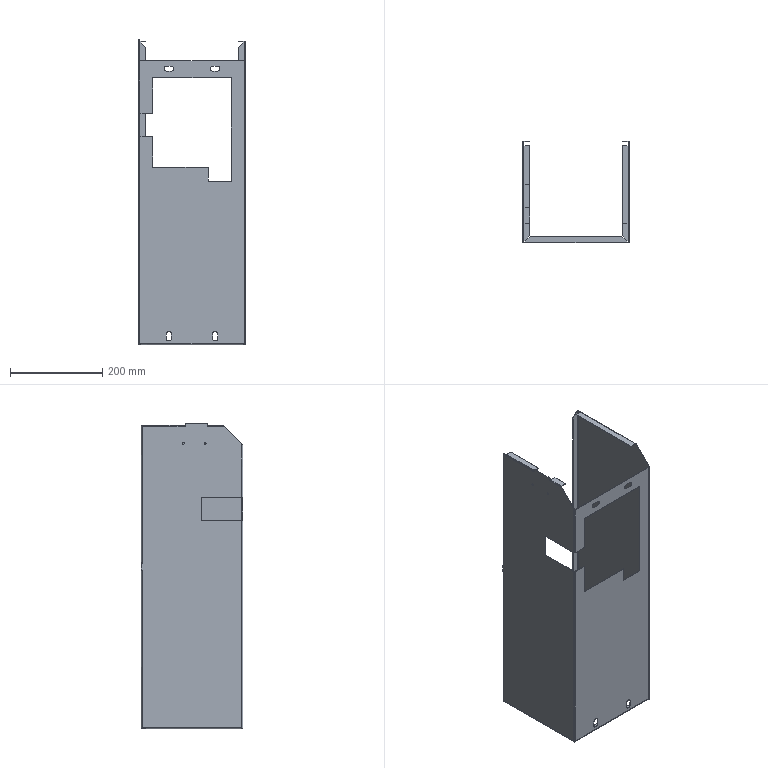Part | SolidWorks | features BaseBody 1 | 1 solid | 191 faces | box 230 x 220 x 663 mm | volume 415128 mm3 | plane 135 | cylinder 44 | spline 12 | commonest cylinder face diameters 4 x17 2 x13 11 x10 16 x4